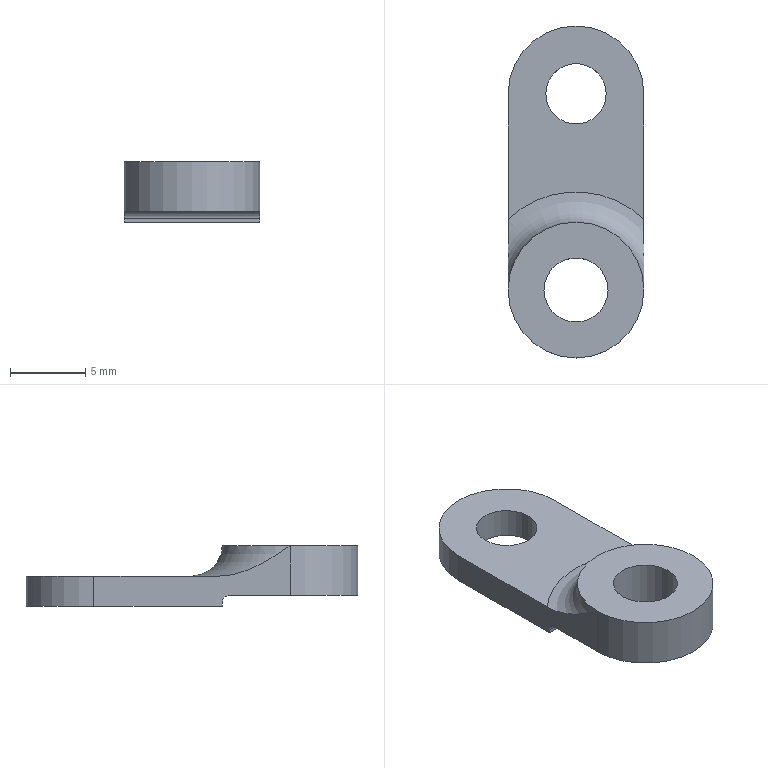NC program | NX | posted with a generic post | part box 9 x 22 x 4 mm
Whole program:
N10 G17 G21 G94 G90
(PLANAR_MILL , TOOL : D10-30-D10-75-3T-FINISH)
N12 T01 M6
N14 G53
N16 G17 G0 G90 X21. Y0. S3500 M3
N18 G43 Z20. H1
N20 Z3.
N22 G94 G1 Z0. F800.
N24 X11.
N26 X-11.
N28 X-21.
N30 Z3.
N32 G0 Z20.
(ADAPTIVE_MILLING , TOOL : D10-30-D10-75-3T-FINISH)
N34 X-6.187 Y-21.55 S4500
N36 Z-3.
N38 G1 X-6.195 Y-21.4 Z-3.937 F2000.
N40 X-6.203 Y-21.25 Z-4.308
N42 X-6.211 Y-21.101 Z-4.58
N44 X-6.219 Y-20.951 Z-4.8
N46 X-6.227 Y-20.801 Z-4.984
N48 X-6.234 Y-20.651 Z-5.142
N50 X-6.242 Y-20.501 Z-5.28
N52 X-6.25 Y-20.352 Z-5.4
N54 X-6.258 Y-20.202 Z-5.505
N56 X-6.266 Y-20.052 Z-5.598
N58 X-6.273 Y-19.902 Z-5.679
N60 X-6.281 Y-19.752 Z-5.75
N62 X-6.289 Y-19.603 Z-5.81
N64 X-6.297 Y-19.453 Z-5.862
N66 X-6.305 Y-19.303 Z-5.905
N68 X-6.312 Y-19.153 Z-5.939
N70 X-6.32 Y-19.003 Z-5.966
N72 X-6.328 Y-18.854 Z-5.985
N74 X-6.336 Y-18.704 Z-5.996
N76 X-6.344 Y-18.554 Z-6.
N78 X-6.429 Y-16.912
N80 G3 X-7.015 Y-16.047 R1.011
N82 X-9.213 Y-15.512 R6.931
N84 X-12.907 Y-15.26 R62.873
N86 G2 X-16.66 Y-12.992 R5.741
N88 X-18.55 Y-8.626 R10.487
N90 X-19.124 Y-2.561 R34.746
N92 X-19.186 Y8.738 R444.893
N94 X-17.032 Y12.554 R5.634
N96 X-12.7 Y14.514 R10.219
N98 X-6.839 Y15.113 R32.434
N100 X5.561 Y15.199 R490.194
N102 G1 X12.76 Y15.184
N104 G2 X16.568 Y13.016 R5.647
N106 X18.497 Y8.775 R10.153
N108 X19.106 Y3.016 R31.399
N110 X19.182 Y-8.783 R360.402
N112 X16.998 Y-12.582 R5.662
N114 X12.655 Y-14.523 R10.268
N116 X6.693 Y-15.117 R33.148
N118 X-4.406 Y-15.177 R314.171
N120 X-10.664 Y-14.59 R385.259
N122 X-15.888 Y-11.053 R7.72
N124 X-17.78 Y-5.921 R13.673
N126 X-18.332 Y0.95 R46.099
N128 X-18.367 Y6.249 R108.3
N130 X-15.257 Y11.611 R7.357
N132 X-10.311 Y13.672 R12.616
N134 X-3.75 Y14.308 R38.815
N136 X10.149 Y14.383 R472.147
N138 X15.611 Y11.262 R7.355
N140 X17.697 Y6.187 R12.726
N142 X18.309 Y-0.276 R39.725
N144 X18.365 Y-6.275 R102.465
N146 X15.297 Y-11.579 R7.345
N148 X10.43 Y-13.644 R12.437
N150 X4.172 Y-14.293 R36.491
N152 X-4.026 Y-14.315 R101.914
N154 X-8.681 Y-13.929 R72.642
N156 X-15.066 Y-9.53 R8.966
N158 X-16.956 Y-4.07 R15.657
N160 X-17.504 Y4.301 R48.293
N162 X-13.664 Y10.792 R8.419
N164 X-8.375 Y12.854 R14.29
N166 X-1.513 Y13.501 R43.109
N168 X8.185 Y13.567 R187.328
N170 X14.841 Y9.616 R8.519
N172 X16.887 Y4.214 R14.626
N174 X17.514 Y-2.951 R46.043
N176 X16.436 Y-7.864 R8.811
N178 X11.971 Y-11.735 R9.631
N180 X6.168 Y-13.192 R19.354
N182 X-6.81 Y-13.242 R63.602
N184 X-14.229 Y-8.202 R9.832
N186 X-16.157 Y-2.344 R17.322
N188 X-16.555 Y2.733 R26.494
N190 X-12.36 Y9.882 R9.036
N192 X-6.886 Y11.999 R15.236
N194 X0.473 Y12.697 R45.648
N196 X6.471 Y12.742 R88.306
N198 X14.099 Y8.083 R9.368
N200 X16.106 Y2.36 R16.343
N202 X16.542 Y-2.712 R25.459
N204 X12.444 Y-9.822 R8.99
N206 X6.883 Y-11.998 R15.139
N208 X-2.177 Y-12.656 R43.548
N210 X-6.648 Y-12.232 R20.956
N212 X-13.348 Y-7.048 R10.386
N214 G3 X-14.115 Y-5.927 R3.598
N216 G1 X-14.923 Y-4.709
N218 X-15.537 Y-3.383
N220 X-15.945 Y-1.98
N222 X-16.135 Y-0.532
N224 X-16.105 Y0.929
N226 G2 X-15.134 Y4.549 R13.787
N228 X-9.908 Y9.74 R10.758
N230 X-3.671 Y11.468 R20.185
N232 X5.01 Y11.889 R56.543
N234 X13.167 Y6.964 R9.938
N236 G1 X13.959 Y6.122
N238 X14.817 Y4.895
N240 X15.473 Y3.549
N242 X15.914 Y2.119
N244 X16.129 Y0.637
N246 X16.111 Y-0.86
N248 G2 X15.145 Y-4.519 R13.778
N250 X9.846 Y-9.766 R10.794
N252 X3.501 Y-11.485 R20.374
N254 X-3.983 Y-11.648 R34.858
N256 X-10.213 Y-8.895 R11.041
N258 G1 X-10.739 Y-8.669
N260 X-11.999 Y-7.93
N262 X-13.133 Y-7.009
N264 X-14.115 Y-5.927
N266 X-14.923 Y-4.709
N268 X-15.537 Y-3.383
N270 X-15.945 Y-1.98
N272 X-16.135 Y-0.532
N274 X-16.105 Y0.929
N276 X-15.855 Y2.369
N278 X-15.39 Y3.754
N280 X-14.724 Y5.049
N282 X-13.87 Y6.229
N284 X-12.848 Y7.268
N286 X-11.682 Y8.141
N288 X-10.397 Y8.828
N290 G2 X-0.782 Y10.859 R34.495
N292 X4.211 Y10.963 R30.129
N294 X8.993 Y9.338 R10.351
N296 G1 X10.52 Y8.773
N298 X11.731 Y8.109
N300 X12.923 Y7.202
N302 X13.269 Y6.841
N304 G3 X14.95 Y7.252 R1.
N306 X14.89 Y7.981 Z-5.962 R1.064
N308 G1 X14.45 Y9.124 Z-5.9
N310 X13.843 Y10.703 F15000.
N312 G3 X13.269 Y11.278 R1.002
N314 X9.239 Y12.786 R121.257
N316 G1 X8.364 Y13.085
N318 X7.483 Y13.364
N320 G3 X3.744 Y13.983 R17.17
N322 X-0.122 Y13.959 R29.672
N324 X-2.873 Y13.683 R43.675
N326 G1 X-6.806 Y13.156
N328 G3 X-7.266 Y12.97 R1.02
N330 G1 X-8.738 Y11.886
N332 X-9.855 Y11.06 Z-5.97 F2000.
N334 G3 X-10.171 Y10.581 Z-6. R1.005
N336 X-9.024 Y9.314 R1.
N338 G2 X-5.867 Y9.665 R12.589
N340 X0.52 Y10.111 R462.036
N342 X5.335 Y9.65 R15.643
N344 X7.878 Y9.551 R19.93
N346 G1 X9.227 Y9.257
N348 G3 X10.289 Y10.762 R1.
N350 X9.895 Y11.129 Z-5.972 R1.139
N352 G1 X8.689 Y11.893 Z-5.9
N354 X7.787 Y12.464 F15000.
N356 G3 X7.286 Y12.618 R1.016
N358 G1 X-4.328 Y13.012
N360 G3 X-4.943 Y12.826 R1.007
N362 G1 X-5.938 Y12.115
N364 X-6.905 Y11.418 Z-5.961 F2000.
N366 G3 X-7.264 Y10.749 Z-6. R1.
N368 X-6.269 Y9.65 R1.
N370 G1 X6.501
N372 G2 X9.227 Y9.257 R11.243
N374 X11.731 Y8.109 R11.24
N376 G1 X12.923 Y7.202
N378 X13.959 Y6.122
N380 X14.817 Y4.895
N382 X15.473 Y3.549
N384 X15.914 Y2.119
N386 X16.129 Y0.637
N388 X16.111 Y-0.86
N390 X15.863 Y-2.337
N392 X15.389 Y-3.757
N394 X14.701 Y-5.086
N396 X13.815 Y-6.294
N398 X12.754 Y-7.349
N400 X11.542 Y-8.228
N402 G2 X8.928 Y-9.348 R11.595
N404 X-2.419 Y-10.802 R32.199
N406 X-6.844 Y-9.645 R12.625
N408 G3 X-7.958 Y-9.539 R10.658
N410 G1 X-9.381 Y-9.21
N412 X-10.311 Y-8.84
N414 G3 X-11.203 Y-10.621 R1.
N416 G1 X-11.068 Y-10.704
N418 X-9.387 Y-11.734 Z-5.9
N420 X-9.071 Y-11.931 F15000.
N422 X-8.748 Y-12.115
N424 X-8.563 Y-12.176
N426 X-8.37 Y-12.201
N428 X7.178 Y-12.65
N430 G3 X7.754 Y-12.487 R1.009
N432 G1 X8.63 Y-11.914
N434 X9.92 Y-11.067 Z-5.978 F2000.
N436 G3 X10.2 Y-10.748 Z-6. R1.022
N438 X9.119 Y-9.288 R1.
N440 G2 X5.976 Y-9.657 R11.853
N442 X0.434 Y-9.964 R177.617
N444 X-3.231 Y-9.65 R17.499
N446 G1 X-6.501
N448 X-6.999 Y-9.612
N450 G3 X-7.326 Y-11.577 R1.
N452 G1 X-7.173 Y-11.617
N454 X-5.265 Y-12.111 Z-5.9
N456 X-4.342 Y-12.346 F15000.
N458 X4.259 Y-13.012
N460 G3 X4.926 Y-12.822 R1.005
N462 G1 X5.879 Y-12.124
N464 X6.844 Y-11.412 Z-5.961 F2000.
N466 G3 X7.195 Y-10.746 Z-6. R1.
N468 X6.199 Y-9.65 R1.
N470 G1 X-3.301
N472 G3 X-4.301 Y-10.798 R1.01
N474 G1 X-4.12 Y-12.115
N476 X-4.099 Y-12.263 Z-5.996
N478 X-4.079 Y-12.412 Z-5.985
N480 X-4.058 Y-12.56 Z-5.966
N482 X-4.038 Y-12.709 Z-5.939
N484 X-4.017 Y-12.858 Z-5.905
N486 X-3.997 Y-13.006 Z-5.862
N488 X-3.976 Y-13.155 Z-5.81
N490 X-3.956 Y-13.303 Z-5.75
N492 X-3.935 Y-13.452 Z-5.679
N494 X-3.915 Y-13.601 Z-5.598
N496 X-3.894 Y-13.749 Z-5.505
N498 X-3.874 Y-13.898 Z-5.4
N500 X-3.853 Y-14.046 Z-5.28
N502 X-3.833 Y-14.195 Z-5.142
N504 X-3.812 Y-14.344 Z-4.984
N506 X-3.792 Y-14.492 Z-4.8
N508 X-3.771 Y-14.641 Z-4.58
N510 X-3.751 Y-14.789 Z-4.308
N512 X-3.73 Y-14.938 Z-3.937
N514 X-3.71 Y-15.087 Z-3.
N516 G0 Z20.
(PLANAR_MILL_1 , TOOL : D10-30-D10-75-3T-FINISH)
N518 X7.7 Y11.5 S3500
N520 Z1.38
N522 G1 Z-0.62 F800.
N524 Y4.5
N526 Y-4.5
N528 Y-11.5
N530 Z1.38
N532 G0 Z20.
N534 M5
(DRILLING , TOOL : 倒角D3-90度)
N536 T02 M6
N538 G53
N540 G17 G0 G90 X-6.5 Y0. S3000 M3
N542 G43 Z20. H2
N544 G94 G81 G99 Z-1.5 F150. R3.
N546 X6.5 Z-2.22 R2.28
N548 G80
N550 G0 X6.5 Y0. Z20.
N552 M5
(DRILLING_1 , TOOL : 钻头D3.8-48-76)
N554 T03 M6
N556 G53
N558 G17 G0 G90 X-6.5 Y0. S3000 M3
N560 G43 Z20. H3
N562 G94 G81 G99 Z-4.642 F150. R3.
N564 X6.5 Z-6.642 R2.28
N566 G80
N568 G0 X6.5 Y0. Z20.
N570 M5
(HOLE_MILLING , TOOL : D2-6-D4-50-3T-FINISH)
N572 T04 M6
N574 G53
N576 G17 G0 G90 X-6.5 Y0. S4500 M3
N578 G43 Z20. H4
N580 Z1.
N582 G94 G3 X-6.988 Y-0.488 R0.487 F600.
N584 X-6.5 Y-0.975 R0.487
N586 X-6.5 Y-0.975 Z0.7 I0. J0.975
N588 X-6.5 Y-0.975 Z0.4 I0. J0.975
N590 X-6.5 Y-0.975 Z0.1 I0. J0.975
N592 X-6.5 Y-0.975 Z-0.2 I0. J0.975
N594 X-6.5 Y-0.975 Z-0.5 I0. J0.975
N596 X-6.5 Y-0.975 Z-0.8 I0. J0.975
N598 X-6.5 Y-0.975 Z-1.1 I0. J0.975
N600 X-6.5 Y-0.975 Z-1.4 I0. J0.975
N602 X-6.5 Y-0.975 Z-1.7 I0. J0.975
N604 X-6.5 Y-0.975 Z-2. I0. J0.975
N606 X-6.5 Y-0.975 Z-2.3 I0. J0.975
N608 X-6.5 Y-0.975 Z-2.6 I0. J0.975
N610 X-6.5 Y-0.975 Z-2.9 I0. J0.975
N612 X-5.656 Y0.488 Z-3. R0.975
N614 X-6.988 Y0.844 R0.975
N616 X-5.656 Y0.488 R-0.975
N618 X-6.322 Y0.666 R0.487
N620 X-6.5 Y0. R0.487
N622 G0 Z20.
N624 X6.5
N626 Z0.28
N628 G3 X6.013 Y-0.488 R0.487
N630 X6.5 Y-0.975 R0.487
N632 X6.5 Y-0.975 Z-0.02 I0. J0.975
N634 X6.5 Y-0.975 Z-0.32 I0. J0.975
N636 X6.5 Y-0.975 Z-0.62 I0. J0.975
N638 X6.5 Y-0.975 Z-0.92 I0. J0.975
N640 X6.5 Y-0.975 Z-1.22 I0. J0.975
N642 X6.5 Y-0.975 Z-1.52 I0. J0.975
N644 X6.5 Y-0.975 Z-1.82 I0. J0.975
N646 X6.5 Y-0.975 Z-2.12 I0. J0.975
N648 X6.5 Y-0.975 Z-2.42 I0. J0.975
N650 X6.5 Y-0.975 Z-2.72 I0. J0.975
N652 X6.5 Y-0.975 Z-3.02 I0. J0.975
N654 X6.5 Y-0.975 Z-3.32 I0. J0.975
N656 X6.5 Y-0.975 Z-3.62 I0. J0.975
N658 X6.5 Y-0.975 Z-3.92 I0. J0.975
N660 X6.5 Y-0.975 Z-4.22 I0. J0.975
N662 X6.5 Y-0.975 Z-4.52 I0. J0.975
N664 X5.656 Y0.488 Z-4.72 R-0.975
N666 X6.013 Y-0.844 R0.975
N668 X5.656 Y0.488 R-0.975
N670 X5.834 Y-0.178 R0.488
N672 X6.5 Y0. R0.488
N674 G0 Z20.
(HOLE_MILLING_COPY , TOOL : D2-6-D4-50-3T-FINISH)
N676 X-6.5
N678 Z-3.
N680 G41 G1 X-6.6 Y-0.003 F300. D4
N682 G3 X-6.5 Y-0.975 R0.491
N684 X-5.525 Y0. R0.975
N686 X-6.5 Y-0.975 R-0.975
N688 X-6.4 Y-0.003 R0.491
N690 G40
N692 G1 X-6.5 Y0.
N694 G0 Z20.
N696 X6.5
N698 Z-4.72
N700 G41 G1 X6.4 Y-0.003
N702 G3 X6.5 Y-0.975 R0.491
N704 X7.475 Y0. R0.975
N706 X6.5 Y-0.975 R-0.975
N708 X6.6 Y-0.003 R0.491
N710 G40
N712 G1 X6.5 Y0.
N714 G0 Z20.
N716 M5
(PLANAR_MILL_2_COPY_COPY , TOOL : D4R0.5)
N718 T05 M6
N720 G53
N722 G17 G0 G90 X4.35 Y8.5 S4500 M3
N724 G43 Z20. H5
N726 Z1.33
N728 G94 G1 Z-0.67 F800.
N730 Y4.5
N732 Y-4.5
N734 Y-8.5
N736 Z1.33
N738 G0 Z20.
N740 X4.25 Y8.5
N742 Z1.33
N744 G1 Z-0.67
N746 Y4.5
N748 Y-4.5
N750 Y-8.5
N752 Z1.33
N754 G0 Z20.
N756 X4.15 Y8.5
N758 Z1.33
N760 G1 Z-0.67
N762 Y4.5
N764 Y-4.5
N766 Y-8.5
N768 Z1.33
N770 G0 Z20.
N772 X4.05 Y8.5
N774 Z1.33
N776 G1 Z-0.67
N778 Y4.5
N780 Y-4.5
N782 Y-8.5
N784 Z1.33
N786 G0 Z20.
(PLANAR_MILL_2_COPY , TOOL : D4R0.5)
N788 X11.2 Y8.5
N790 Z1.28
N792 G1 Z-0.72
N794 Y4.5
N796 Y-4.5
N798 Y-8.5
N800 Z1.28
N802 G0 Z20.
N804 X8.8 Y8.5
N806 Z1.28
N808 G1 Z-0.72
N810 Y4.5
N812 Y-4.5
N814 Y-8.5
N816 Z1.28
N818 G0 Z20.
N820 X6.4 Y8.5
N822 Z1.28
N824 G1 Z-0.72
N826 Y4.5
N828 Y-4.5
N830 Y-8.5
N832 Z1.28
N834 G0 Z20.
N836 X4. Y8.5
N838 Z1.28
N840 G1 Z-0.72
N842 Y4.5
N844 Y-4.5
N846 Y-8.5
N848 Z1.28
N850 G0 Z20.
(PLANAR_MILL_2 , TOOL : D4R0.5)
N852 X8.5
N854 Z-4.
N856 G1 Z-6.
N858 G3 X6.5 Y-6.5 R2.
N860 G1 X-6.5
N862 G2 X-13. Y0. R6.5
N864 X-6.5 Y6.5 R6.5
N866 G1 X6.5
N868 G2 X13. Y0. R6.5
N870 X6.5 Y-6.5 R6.5
N872 G3 X4.5 Y-8.5 R2.
N874 G1 X8.5
N876 G3 X6.5 Y-6.5 R2.
N878 G1 X-6.5
N880 G2 X-13. Y0. R6.5
N882 X-6.5 Y6.5 R6.5
N884 G1 X6.5
N886 G2 X13. Y0. R6.5
N888 X6.5 Y-6.5 R6.5
N890 G3 X4.5 Y-8.5 R2.
N892 G1 Z-4.
N894 G0 Z20.
N896 M5
(PLANAR_MILL_3 , TOOL : 球刀R0.5-2-D4-50)
N898 T06 M6
N900 G53
N902 G17 G0 G90 X-1.25 Y-5.9 S4500 M3
N904 G43 Z20. H6
N906 Z1.8
N908 G94 G1 Z-0.2 F800.
N910 G3 X-2.25 Y-4.9 R1.
N912 G1 X-6.5
N914 G2 X-11.4 Y0. R4.9
N916 X-6.5 Y4.9 R4.9
N918 G1 X2.
N920 G2 X2.4 Y4.5 R0.4
N922 G1 Y-4.5
N924 G2 X2. Y-4.9 R0.4
N926 G1 X-2.25
N928 G3 X-3.25 Y-5.9 R1.
N930 G1 Z1.8
N932 G0 Z20.
(PLANAR_MILL_3_COPY , TOOL : 球刀R0.5-2-D4-50)
N934 X-7. Y-0.98
N936 Z1.8
N938 G1 Z-0.2
N940 Y-1.1
N942 G3 X-6.5 Y-1.6 R0.5
N944 X-4.9 Y0. R1.6
N946 X-6.5 Y-1.6 R-1.6
N948 X-6. Y-1.1 R0.5
N950 G1 Y-0.98
N952 Z1.8
N954 G0 Z20.
(PLANAR_MILL_3_COPY_1 , TOOL : 球刀R0.5-2-D4-50)
N956 X2.8 Y5.1
N958 Z1.08
N960 G1 Z-0.92
N962 G3 X3. Y4.9 R0.2
N964 G1 X6.5
N966 G2 X11.4 Y0. R4.9
N968 X6.5 Y-4.9 R4.9
N970 G1 X3.
N972 G3 X2.8 Y-5.1 R0.2
N974 G1 Z1.08
N976 G0 Z20.
(PLANAR_MILL_3_COPY_COPY , TOOL : 球刀R0.5-2-D4-50)
N978 X6. Y-1.118
N980 Z1.08
N982 G1 Z-0.92
N984 Y-1.225
N986 G3 X6.5 Y-1.725 R0.5
N988 X8.225 Y0. R1.725
N990 X6.5 Y-1.725 R-1.725
N992 X7. Y-1.225 R0.5
N994 G1 Y-1.118
N996 Z1.08
N998 G0 Z20.
N1000 M5
N1002 M2